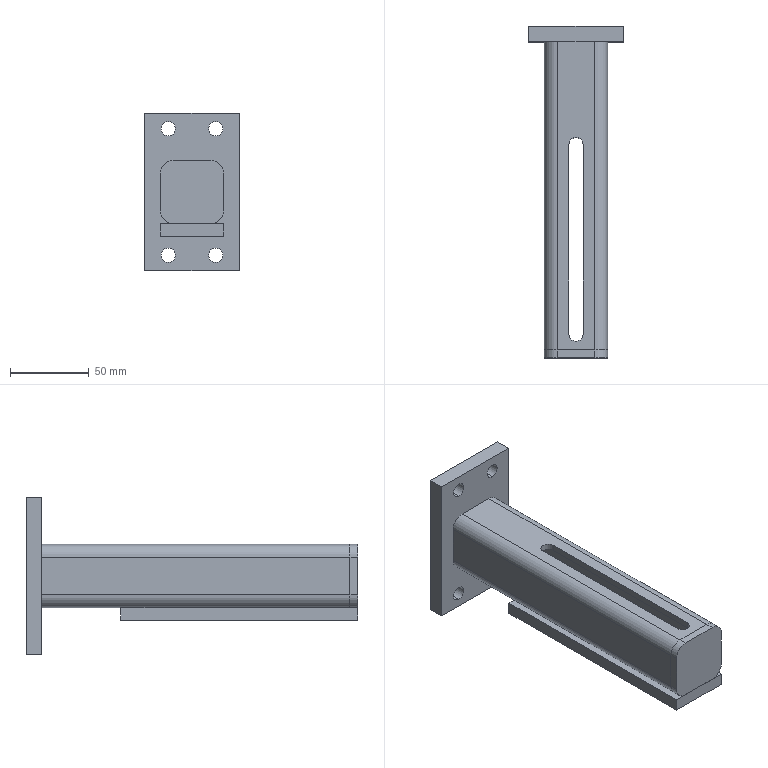Part | SolidWorks | features ICE 3, EndCap 1, HoleWzd 1, WeldMemberFeat 1, WeldmentFeature 1 | 4 solids | 60 faces | box 60 x 210 x 100 mm | volume 199168 mm3 | plane 34 | cylinder 26 | commonest cylinder face diameters 9 x14 16 x8 8 x4